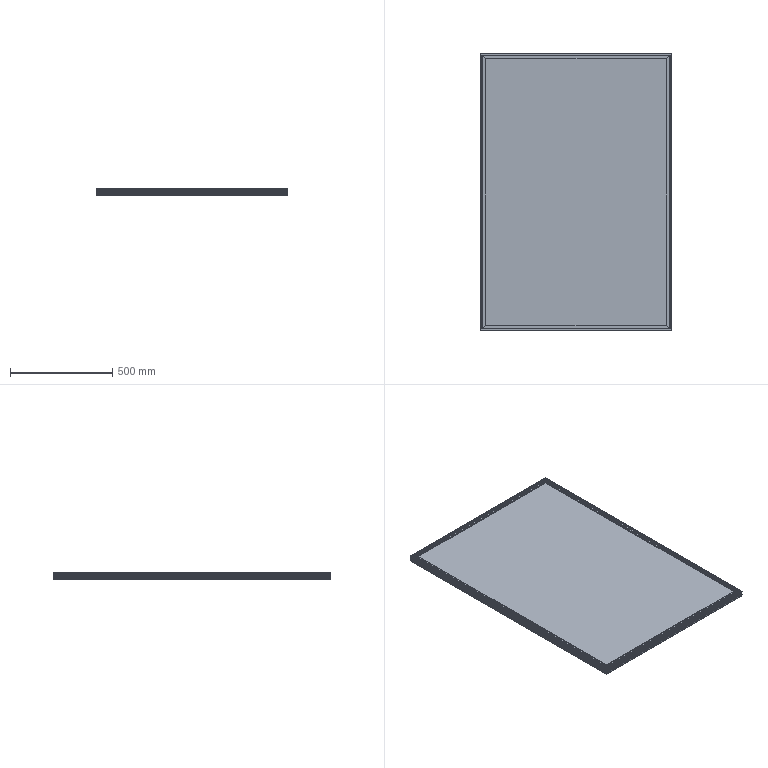Part | SolidWorks | features ICE 1, WeldMemberFeat 1, WeldmentFeature 1 | 5 solids | 272 faces | box 940 x 1360 x 30 mm | volume 20874219 mm3 | plane 222 | cylinder 50 | commonest cylinder face diameters 0.4 x26 2 x16 1 x8